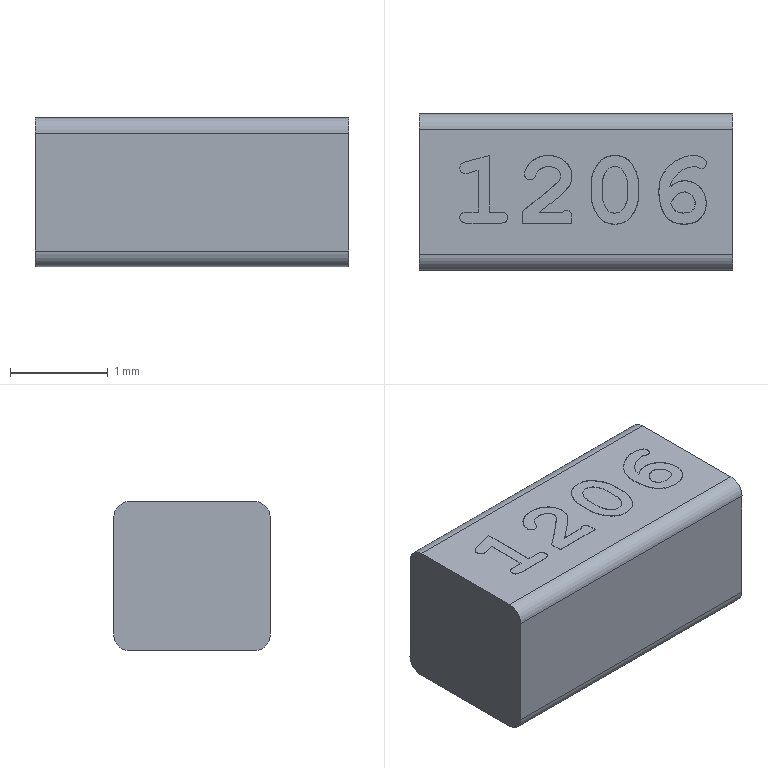Part | STEP file | RJ-USIO-V1_2-220411_100 | 1 solid | 81 faces | box 3.2 x 1.6 x 1.527 mm | volume 7.736 mm3 | cylinder 28 | plane 27 | other 26 | commonest cylinder face diameters 0.32 x4 0.107 x3 0.114 x2 0.194 x2 0.198 x2 0.111 x1